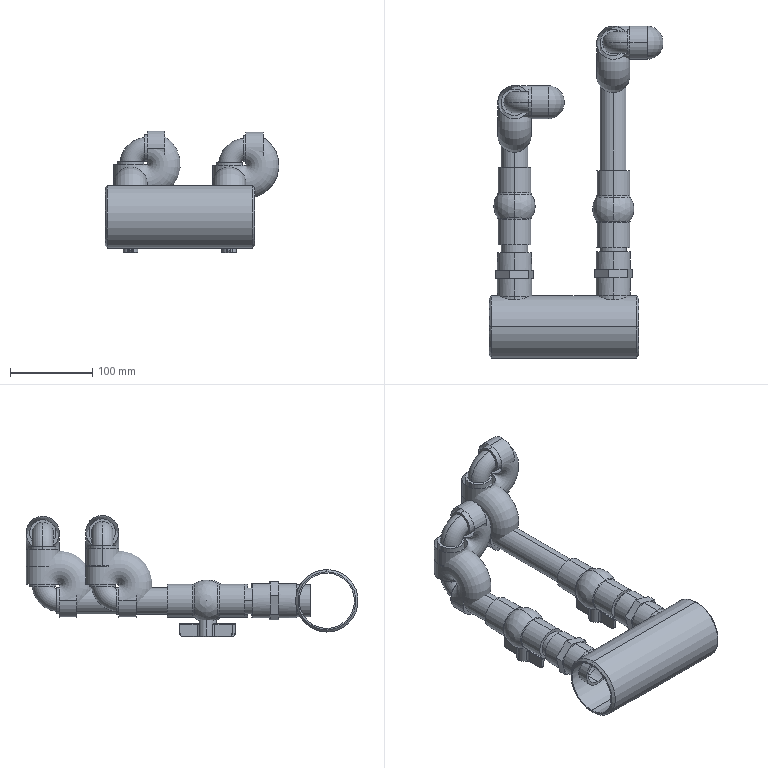Part | SolidWorks | features MoveCopyBody 11, Stock 10, ICE 6, Chamfer 1, WeldMemberFeat 1, WeldmentFeature 1 | 19 solids | 376 faces | box 211.75 x 403.566 x 147.274 mm | volume 1044578 mm3 | cylinder 158 | plane 104 | torus 62 | sphere 28 | cone 16 | spline 8 | commonest cylinder face diameters 0.508 x30 32 x30 40.5 x16 5.723 x12 25.4 x12 32.004 x10